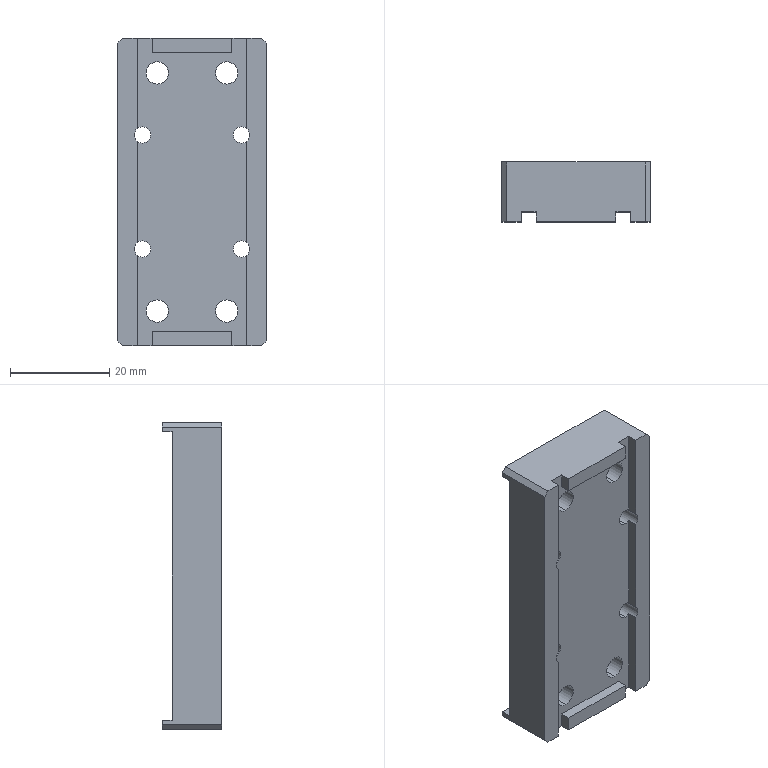Part | SolidWorks | features ICE 3, HoleWzd 2, Chamfer 1, Extrusion 1, MirrorPattern 1 | 1 solid | 58 faces | box 30 x 12 x 62 mm | volume 15056 mm3 | plane 34 | cylinder 24 | commonest cylinder face diameters 3.3 x8 4.5 x8 8 x8